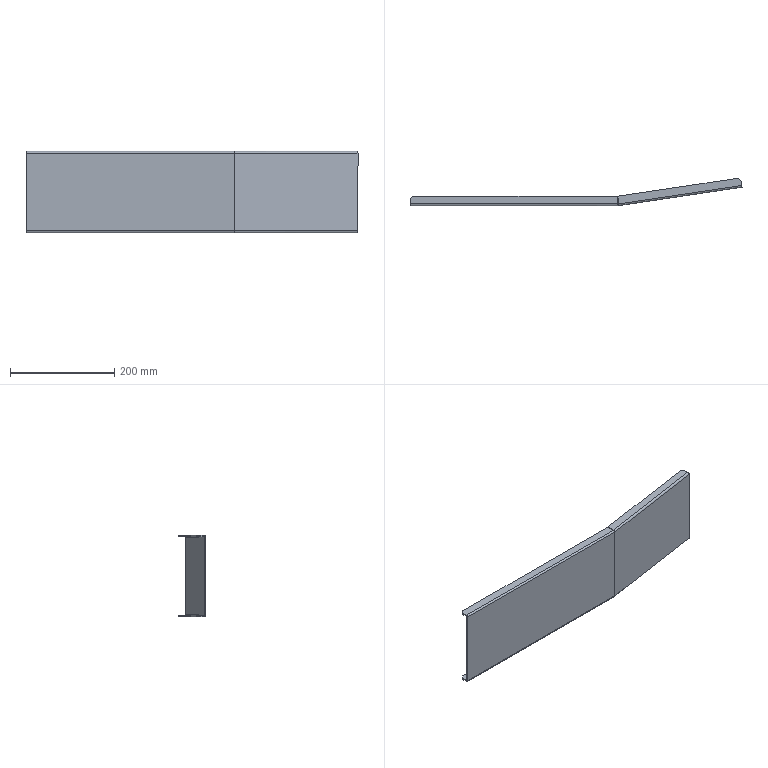Part | SolidWorks | features Chamfer 1, EdgeFlange 1, FlatPattern 1, SMBaseFlange 1, SheetMetal 1 | 1 solid | 54 faces | box 637.807 x 52.57 x 156 mm | volume 354234 mm3 | plane 40 | cylinder 10 | spline 4 | commonest cylinder face diameters 0.2 x4 6.2 x4 2 x1 8 x1